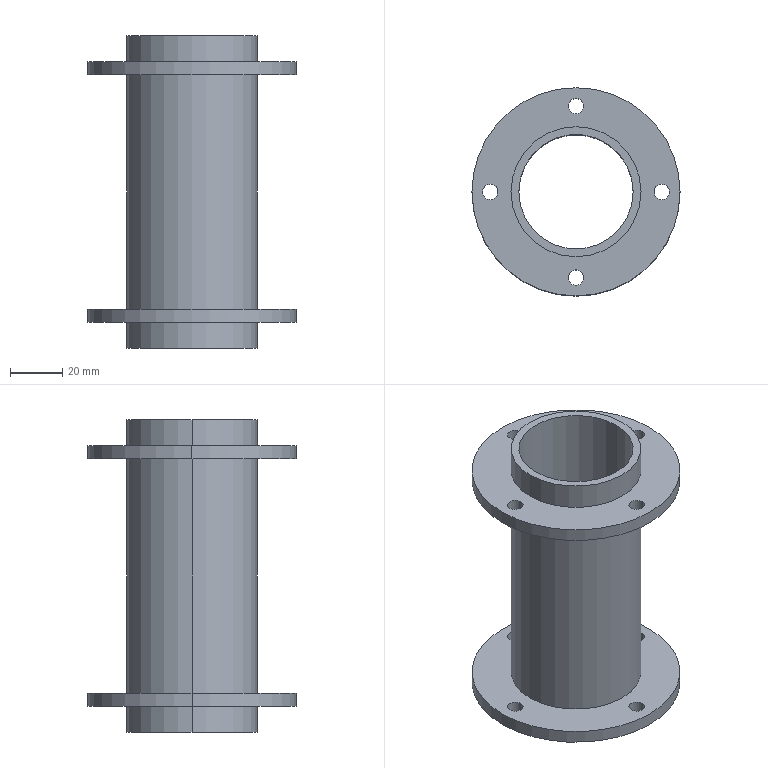Part | SolidWorks | features Extrusion 1, ICE 1, MirrorPattern 1 | 1 solid | 34 faces | box 80 x 80 x 120 mm | volume 82655 mm3 | cylinder 28 | plane 6 | commonest cylinder face diameters 6 x16 50 x6 80 x4 44 x2
STEP:
#1=CARTESIAN_POINT('',(36.,0.,45.));
#2=VERTEX_POINT('',#1);
#3=CARTESIAN_POINT('',(30.,0.,45.));
#4=VERTEX_POINT('',#3);
#5=CARTESIAN_POINT('',(33.,0.,45.));
#6=DIRECTION('',(0.,0.,-1.));
#7=DIRECTION('',(-1.,0.,0.));
#8=AXIS2_PLACEMENT_3D('',#5,#6,#7);
#9=CIRCLE('',#8,3.);
#10=EDGE_CURVE('',#2,#4,#9,.T.);
#11=ORIENTED_EDGE('',*,*,#10,.T.);
#12=CARTESIAN_POINT('',(30.,0.,50.));
#13=VERTEX_POINT('',#12);
#14=CARTESIAN_POINT('',(30.,0.,45.));
#15=DIRECTION('',(0.,0.,1.));
#16=VECTOR('',#15,1000.);
#17=LINE('',#14,#16);
#18=EDGE_CURVE('',#4,#13,#17,.T.);
#19=ORIENTED_EDGE('',*,*,#18,.T.);
#20=CARTESIAN_POINT('',(36.,0.,50.));
#21=VERTEX_POINT('',#20);
#22=CARTESIAN_POINT('',(33.,0.,50.));
#23=DIRECTION('',(0.,0.,-1.));
#24=DIRECTION('',(-1.,0.,0.));
#25=AXIS2_PLACEMENT_3D('',#22,#23,#24);
#26=CIRCLE('',#25,3.);
#27=EDGE_CURVE('',#21,#13,#26,.T.);
#28=ORIENTED_EDGE('',*,*,#27,.F.);
#29=CARTESIAN_POINT('',(36.,0.,45.));
#30=DIRECTION('',(0.,0.,1.));
#31=VECTOR('',#30,1000.);
#32=LINE('',#29,#31);
#33=EDGE_CURVE('',#2,#21,#32,.T.);
#34=ORIENTED_EDGE('',*,*,#33,.F.);
#35=EDGE_LOOP('',(#11,#19,#28,#34));
#36=FACE_OUTER_BOUND('',#35,.T.);
#37=CARTESIAN_POINT('',(33.,0.,45.));
#38=DIRECTION('',(0.,0.,1.));
#39=DIRECTION('',(1.,0.,0.));
#40=AXIS2_PLACEMENT_3D('',#37,#38,#39);
#41=CYLINDRICAL_SURFACE('',#40,3.);
#42=ADVANCED_FACE('',(#36),#41,.F.);
#43=CARTESIAN_POINT('',(3.,-33.,45.));
#44=VERTEX_POINT('',#43);
#45=CARTESIAN_POINT('',(-3.,-33.,45.));
#46=VERTEX_POINT('',#45);
#47=CARTESIAN_POINT('',(0.,-33.,45.));
#48=DIRECTION('',(0.,0.,-1.));
#49=DIRECTION('',(-1.,0.,0.));
#50=AXIS2_PLACEMENT_3D('',#47,#48,#49);
#51=CIRCLE('',#50,3.);
#52=EDGE_CURVE('',#44,#46,#51,.T.);
#53=ORIENTED_EDGE('',*,*,#52,.T.);
#54=CARTESIAN_POINT('',(-3.,-33.,50.));
#55=VERTEX_POINT('',#54);
#56=CARTESIAN_POINT('',(-3.,-33.,45.));
#57=DIRECTION('',(0.,0.,1.));
#58=VECTOR('',#57,1000.);
#59=LINE('',#56,#58);
#60=EDGE_CURVE('',#46,#55,#59,.T.);
#61=ORIENTED_EDGE('',*,*,#60,.T.);
#62=CARTESIAN_POINT('',(3.,-33.,50.));
#63=VERTEX_POINT('',#62);
#64=CARTESIAN_POINT('',(0.,-33.,50.));
#65=DIRECTION('',(0.,0.,-1.));
#66=DIRECTION('',(-1.,0.,0.));
#67=AXIS2_PLACEMENT_3D('',#64,#65,#66);
#68=CIRCLE('',#67,3.);
#69=EDGE_CURVE('',#63,#55,#68,.T.);
#70=ORIENTED_EDGE('',*,*,#69,.F.);
#71=CARTESIAN_POINT('',(3.,-33.,45.));
#72=DIRECTION('',(0.,0.,1.));
#73=VECTOR('',#72,1000.);
#74=LINE('',#71,#73);
#75=EDGE_CURVE('',#44,#63,#74,.T.);
#76=ORIENTED_EDGE('',*,*,#75,.F.);
#77=EDGE_LOOP('',(#53,#61,#70,#76));
#78=FACE_OUTER_BOUND('',#77,.T.);
#79=CARTESIAN_POINT('',(0.,-33.,45.));
#80=DIRECTION('',(0.,0.,1.));
#81=DIRECTION('',(1.,0.,0.));
#82=AXIS2_PLACEMENT_3D('',#79,#80,#81);
#83=CYLINDRICAL_SURFACE('',#82,3.);
#84=ADVANCED_FACE('',(#78),#83,.F.);
#85=CARTESIAN_POINT('',(-30.,0.,45.));
#86=VERTEX_POINT('',#85);
#87=CARTESIAN_POINT('',(-36.,0.,45.));
#88=VERTEX_POINT('',#87);
#89=CARTESIAN_POINT('',(-33.,0.,45.));
#90=DIRECTION('',(0.,0.,-1.));
#91=DIRECTION('',(-1.,0.,0.));
#92=AXIS2_PLACEMENT_3D('',#89,#90,#91);
#93=CIRCLE('',#92,3.);
#94=EDGE_CURVE('',#86,#88,#93,.T.);
#95=ORIENTED_EDGE('',*,*,#94,.T.);
#96=CARTESIAN_POINT('',(-36.,0.,50.));
#97=VERTEX_POINT('',#96);
#98=CARTESIAN_POINT('',(-36.,0.,45.));
#99=DIRECTION('',(0.,0.,1.));
#100=VECTOR('',#99,1000.);
#101=LINE('',#98,#100);
#102=EDGE_CURVE('',#88,#97,#101,.T.);
#103=ORIENTED_EDGE('',*,*,#102,.T.);
#104=CARTESIAN_POINT('',(-30.,0.,50.));
#105=VERTEX_POINT('',#104);
#106=CARTESIAN_POINT('',(-33.,0.,50.));
#107=DIRECTION('',(0.,0.,-1.));
#108=DIRECTION('',(-1.,0.,0.));
#109=AXIS2_PLACEMENT_3D('',#106,#107,#108);
#110=CIRCLE('',#109,3.);
#111=EDGE_CURVE('',#105,#97,#110,.T.);
#112=ORIENTED_EDGE('',*,*,#111,.F.);
#113=CARTESIAN_POINT('',(-30.,0.,45.));
#114=DIRECTION('',(0.,0.,1.));
#115=VECTOR('',#114,1000.);
#116=LINE('',#113,#115);
#117=EDGE_CURVE('',#86,#105,#116,.T.);
#118=ORIENTED_EDGE('',*,*,#117,.F.);
#119=EDGE_LOOP('',(#95,#103,#112,#118));
#120=FACE_OUTER_BOUND('',#119,.T.);
#121=CARTESIAN_POINT('',(-33.,0.,45.));
#122=DIRECTION('',(0.,0.,1.));
#123=DIRECTION('',(1.,0.,0.));
#124=AXIS2_PLACEMENT_3D('',#121,#122,#123);
#125=CYLINDRICAL_SURFACE('',#124,3.);
#126=ADVANCED_FACE('',(#120),#125,.F.);
#127=CARTESIAN_POINT('',(3.,33.,45.));
#128=VERTEX_POINT('',#127);
#129=CARTESIAN_POINT('',(-3.,33.,45.));
#130=VERTEX_POINT('',#129);
#131=CARTESIAN_POINT('',(0.,33.,45.));
#132=DIRECTION('',(0.,0.,-1.));
#133=DIRECTION('',(-1.,0.,0.));
#134=AXIS2_PLACEMENT_3D('',#131,#132,#133);
#135=CIRCLE('',#134,3.);
#136=EDGE_CURVE('',#128,#130,#135,.T.);
#137=ORIENTED_EDGE('',*,*,#136,.T.);
#138=CARTESIAN_POINT('',(-3.,33.,50.));
#139=VERTEX_POINT('',#138);
#140=CARTESIAN_POINT('',(-3.,33.,45.));
#141=DIRECTION('',(0.,0.,1.));
#142=VECTOR('',#141,1000.);
#143=LINE('',#140,#142);
#144=EDGE_CURVE('',#130,#139,#143,.T.);
#145=ORIENTED_EDGE('',*,*,#144,.T.);
#146=CARTESIAN_POINT('',(3.,33.,50.));
#147=VERTEX_POINT('',#146);
#148=CARTESIAN_POINT('',(0.,33.,50.));
#149=DIRECTION('',(0.,0.,-1.));
#150=DIRECTION('',(-1.,0.,0.));
#151=AXIS2_PLACEMENT_3D('',#148,#149,#150);
#152=CIRCLE('',#151,3.);
#153=EDGE_CURVE('',#147,#139,#152,.T.);
#154=ORIENTED_EDGE('',*,*,#153,.F.);
#155=CARTESIAN_POINT('',(3.,33.,45.));
#156=DIRECTION('',(0.,0.,1.));
#157=VECTOR('',#156,1000.);
#158=LINE('',#155,#157);
#159=EDGE_CURVE('',#128,#147,#158,.T.);
#160=ORIENTED_EDGE('',*,*,#159,.F.);
#161=EDGE_LOOP('',(#137,#145,#154,#160));
#162=FACE_OUTER_BOUND('',#161,.T.);
#163=CARTESIAN_POINT('',(0.,33.,45.));
#164=DIRECTION('',(0.,0.,1.));
#165=DIRECTION('',(1.,0.,0.));
#166=AXIS2_PLACEMENT_3D('',#163,#164,#165);
#167=CYLINDRICAL_SURFACE('',#166,3.);
#168=ADVANCED_FACE('',(#162),#167,.F.);
#169=CARTESIAN_POINT('',(-40.,0.,45.));
#170=VERTEX_POINT('',#169);
#171=CARTESIAN_POINT('',(40.,0.,45.));
#172=VERTEX_POINT('',#171);
#173=CARTESIAN_POINT('',(0.,0.,45.));
#174=DIRECTION('',(0.,0.,-1.));
#175=DIRECTION('',(-1.,0.,0.));
#176=AXIS2_PLACEMENT_3D('',#173,#174,#175);
#177=CIRCLE('',#176,40.);
#178=EDGE_CURVE('',#170,#172,#177,.T.);
#179=ORIENTED_EDGE('',*,*,#178,.F.);
#180=CARTESIAN_POINT('',(-40.,0.,50.));
#181=VERTEX_POINT('',#180);
#182=CARTESIAN_POINT('',(-40.,0.,45.));
#183=DIRECTION('',(0.,0.,1.));
#184=VECTOR('',#183,1000.);
#185=LINE('',#182,#184);
#186=EDGE_CURVE('',#170,#181,#185,.T.);
#187=ORIENTED_EDGE('',*,*,#186,.T.);
#188=CARTESIAN_POINT('',(40.,0.,50.));
#189=VERTEX_POINT('',#188);
#190=CARTESIAN_POINT('',(0.,0.,50.));
#191=DIRECTION('',(0.,0.,-1.));
#192=DIRECTION('',(-1.,0.,0.));
#193=AXIS2_PLACEMENT_3D('',#190,#191,#192);
#194=CIRCLE('',#193,40.);
#195=EDGE_CURVE('',#181,#189,#194,.T.);
#196=ORIENTED_EDGE('',*,*,#195,.T.);
#197=CARTESIAN_POINT('',(40.,0.,45.));
#198=DIRECTION('',(0.,0.,1.));
#199=VECTOR('',#198,1000.);
#200=LINE('',#197,#199);
#201=EDGE_CURVE('',#172,#189,#200,.T.);
#202=ORIENTED_EDGE('',*,*,#201,.F.);
#203=EDGE_LOOP('',(#179,#187,#196,#202));
#204=FACE_OUTER_BOUND('',#203,.T.);
#205=CARTESIAN_POINT('',(0.,0.,45.));
#206=DIRECTION('',(0.,0.,1.));
#207=DIRECTION('',(1.,0.,0.));
#208=AXIS2_PLACEMENT_3D('',#205,#206,#207);
#209=CYLINDRICAL_SURFACE('',#208,40.);
#210=ADVANCED_FACE('',(#204),#209,.T.);
#211=CARTESIAN_POINT('',(36.,0.,-45.));
#212=VERTEX_POINT('',#211);
#213=CARTESIAN_POINT('',(30.,0.,-45.));
#214=VERTEX_POINT('',#213);
#215=CARTESIAN_POINT('',(33.,0.,-45.));
#216=DIRECTION('',(0.,0.,-1.));
#217=DIRECTION('',(-1.,0.,0.));
#218=AXIS2_PLACEMENT_3D('',#215,#216,#217);
#219=CIRCLE('',#218,3.);
#220=EDGE_CURVE('',#212,#214,#219,.T.);
#221=ORIENTED_EDGE('',*,*,#220,.F.);
#222=CARTESIAN_POINT('',(36.,0.,-50.));
#223=VERTEX_POINT('',#222);
#224=CARTESIAN_POINT('',(36.,0.,-45.));
#225=DIRECTION('',(0.,0.,-1.));
#226=VECTOR('',#225,1000.);
#227=LINE('',#224,#226);
#228=EDGE_CURVE('',#212,#223,#227,.T.);
#229=ORIENTED_EDGE('',*,*,#228,.T.);
#230=CARTESIAN_POINT('',(30.,0.,-50.));
#231=VERTEX_POINT('',#230);
#232=CARTESIAN_POINT('',(33.,0.,-50.));
#233=DIRECTION('',(0.,0.,-1.));
#234=DIRECTION('',(-1.,0.,0.));
#235=AXIS2_PLACEMENT_3D('',#232,#233,#234);
#236=CIRCLE('',#235,3.);
#237=EDGE_CURVE('',#223,#231,#236,.T.);
#238=ORIENTED_EDGE('',*,*,#237,.T.);
#239=CARTESIAN_POINT('',(30.,0.,-45.));
#240=DIRECTION('',(0.,0.,-1.));
#241=VECTOR('',#240,1000.);
#242=LINE('',#239,#241);
#243=EDGE_CURVE('',#214,#231,#242,.T.);
#244=ORIENTED_EDGE('',*,*,#243,.F.);
#245=EDGE_LOOP('',(#221,#229,#238,#244));
#246=FACE_OUTER_BOUND('',#245,.T.);
#247=CARTESIAN_POINT('',(33.,0.,-45.));
#248=DIRECTION('',(0.,0.,-1.));
#249=DIRECTION('',(-1.,0.,0.));
#250=AXIS2_PLACEMENT_3D('',#247,#248,#249);
#251=CYLINDRICAL_SURFACE('',#250,3.);
#252=ADVANCED_FACE('',(#246),#251,.F.);
#253=CARTESIAN_POINT('',(3.,-33.,-45.));
#254=VERTEX_POINT('',#253);
#255=CARTESIAN_POINT('',(-3.,-33.,-45.));
#256=VERTEX_POINT('',#255);
#257=CARTESIAN_POINT('',(0.,-33.,-45.));
#258=DIRECTION('',(0.,0.,-1.));
#259=DIRECTION('',(-1.,0.,0.));
#260=AXIS2_PLACEMENT_3D('',#257,#258,#259);
#261=CIRCLE('',#260,3.);
#262=EDGE_CURVE('',#254,#256,#261,.T.);
#263=ORIENTED_EDGE('',*,*,#262,.F.);
#264=CARTESIAN_POINT('',(3.,-33.,-50.));
#265=VERTEX_POINT('',#264);
#266=CARTESIAN_POINT('',(3.,-33.,-45.));
#267=DIRECTION('',(0.,0.,-1.));
#268=VECTOR('',#267,1000.);
#269=LINE('',#266,#268);
#270=EDGE_CURVE('',#254,#265,#269,.T.);
#271=ORIENTED_EDGE('',*,*,#270,.T.);
#272=CARTESIAN_POINT('',(-3.,-33.,-50.));
#273=VERTEX_POINT('',#272);
#274=CARTESIAN_POINT('',(0.,-33.,-50.));
#275=DIRECTION('',(0.,0.,-1.));
#276=DIRECTION('',(-1.,0.,0.));
#277=AXIS2_PLACEMENT_3D('',#274,#275,#276);
#278=CIRCLE('',#277,3.);
#279=EDGE_CURVE('',#265,#273,#278,.T.);
#280=ORIENTED_EDGE('',*,*,#279,.T.);
#281=CARTESIAN_POINT('',(-3.,-33.,-45.));
#282=DIRECTION('',(0.,0.,-1.));
#283=VECTOR('',#282,1000.);
#284=LINE('',#281,#283);
#285=EDGE_CURVE('',#256,#273,#284,.T.);
#286=ORIENTED_EDGE('',*,*,#285,.F.);
#287=EDGE_LOOP('',(#263,#271,#280,#286));
#288=FACE_OUTER_BOUND('',#287,.T.);
#289=CARTESIAN_POINT('',(0.,-33.,-45.));
#290=DIRECTION('',(0.,0.,-1.));
#291=DIRECTION('',(-1.,0.,0.));
#292=AXIS2_PLACEMENT_3D('',#289,#290,#291);
#293=CYLINDRICAL_SURFACE('',#292,3.);
#294=ADVANCED_FACE('',(#288),#293,.F.);
#295=CARTESIAN_POINT('',(-30.,0.,-45.));
#296=VERTEX_POINT('',#295);
#297=CARTESIAN_POINT('',(-36.,0.,-45.));
#298=VERTEX_POINT('',#297);
#299=CARTESIAN_POINT('',(-33.,0.,-45.));
#300=DIRECTION('',(0.,0.,-1.));
#301=DIRECTION('',(-1.,0.,0.));
#302=AXIS2_PLACEMENT_3D('',#299,#300,#301);
#303=CIRCLE('',#302,3.);
#304=EDGE_CURVE('',#296,#298,#303,.T.);
#305=ORIENTED_EDGE('',*,*,#304,.F.);
#306=CARTESIAN_POINT('',(-30.,0.,-50.));
#307=VERTEX_POINT('',#306);
#308=CARTESIAN_POINT('',(-30.,0.,-45.));
#309=DIRECTION('',(0.,0.,-1.));
#310=VECTOR('',#309,1000.);
#311=LINE('',#308,#310);
#312=EDGE_CURVE('',#296,#307,#311,.T.);
#313=ORIENTED_EDGE('',*,*,#312,.T.);
#314=CARTESIAN_POINT('',(-36.,0.,-50.));
#315=VERTEX_POINT('',#314);
#316=CARTESIAN_POINT('',(-33.,0.,-50.));
#317=DIRECTION('',(0.,0.,-1.));
#318=DIRECTION('',(-1.,0.,0.));
#319=AXIS2_PLACEMENT_3D('',#316,#317,#318);
#320=CIRCLE('',#319,3.);
#321=EDGE_CURVE('',#307,#315,#320,.T.);
#322=ORIENTED_EDGE('',*,*,#321,.T.);
#323=CARTESIAN_POINT('',(-36.,0.,-45.));
#324=DIRECTION('',(0.,0.,-1.));
#325=VECTOR('',#324,1000.);
#326=LINE('',#323,#325);
#327=EDGE_CURVE('',#298,#315,#326,.T.);
#328=ORIENTED_EDGE('',*,*,#327,.F.);
#329=EDGE_LOOP('',(#305,#313,#322,#328));
#330=FACE_OUTER_BOUND('',#329,.T.);
#331=CARTESIAN_POINT('',(-33.,0.,-45.));
#332=DIRECTION('',(0.,0.,-1.));
#333=DIRECTION('',(-1.,0.,0.));
#334=AXIS2_PLACEMENT_3D('',#331,#332,#333);
#335=CYLINDRICAL_SURFACE('',#334,3.);
#336=ADVANCED_FACE('',(#330),#335,.F.);
#337=CARTESIAN_POINT('',(3.,33.,-45.));
#338=VERTEX_POINT('',#337);
#339=CARTESIAN_POINT('',(-3.,33.,-45.));
#340=VERTEX_POINT('',#339);
#341=CARTESIAN_POINT('',(0.,33.,-45.));
#342=DIRECTION('',(0.,0.,-1.));
#343=DIRECTION('',(-1.,0.,0.));
#344=AXIS2_PLACEMENT_3D('',#341,#342,#343);
#345=CIRCLE('',#344,3.);
#346=EDGE_CURVE('',#338,#340,#345,.T.);
#347=ORIENTED_EDGE('',*,*,#346,.F.);
#348=CARTESIAN_POINT('',(3.,33.,-50.));
#349=VERTEX_POINT('',#348);
#350=CARTESIAN_POINT('',(3.,33.,-45.));
#351=DIRECTION('',(0.,0.,-1.));
#352=VECTOR('',#351,1000.);
#353=LINE('',#350,#352);
#354=EDGE_CURVE('',#338,#349,#353,.T.);
#355=ORIENTED_EDGE('',*,*,#354,.T.);
#356=CARTESIAN_POINT('',(-3.,33.,-50.));
#357=VERTEX_POINT('',#356);
#358=CARTESIAN_POINT('',(0.,33.,-50.));
#359=DIRECTION('',(0.,0.,-1.));
#360=DIRECTION('',(-1.,0.,0.));
#361=AXIS2_PLACEMENT_3D('',#358,#359,#360);
#362=CIRCLE('',#361,3.);
#363=EDGE_CURVE('',#349,#357,#362,.T.);
#364=ORIENTED_EDGE('',*,*,#363,.T.);
#365=CARTESIAN_POINT('',(-3.,33.,-45.));
#366=DIRECTION('',(0.,0.,-1.));
#367=VECTOR('',#366,1000.);
#368=LINE('',#365,#367);
#369=EDGE_CURVE('',#340,#357,#368,.T.);
#370=ORIENTED_EDGE('',*,*,#369,.F.);
#371=EDGE_LOOP('',(#347,#355,#364,#370));
#372=FACE_OUTER_BOUND('',#371,.T.);
#373=CARTESIAN_POINT('',(0.,33.,-45.));
#374=DIRECTION('',(0.,0.,-1.));
#375=DIRECTION('',(-1.,0.,0.));
#376=AXIS2_PLACEMENT_3D('',#373,#374,#375);
#377=CYLINDRICAL_SURFACE('',#376,3.);
#378=ADVANCED_FACE('',(#372),#377,.F.);
#379=CARTESIAN_POINT('',(-40.,0.,-45.));
#380=VERTEX_POINT('',#379);
#381=CARTESIAN_POINT('',(40.,0.,-45.));
#382=VERTEX_POINT('',#381);
#383=CARTESIAN_POINT('',(0.,0.,-45.));
#384=DIRECTION('',(0.,0.,-1.));
#385=DIRECTION('',(-1.,0.,0.));
#386=AXIS2_PLACEMENT_3D('',#383,#384,#385);
#387=CIRCLE('',#386,40.);
#388=EDGE_CURVE('',#380,#382,#387,.T.);
#389=ORIENTED_EDGE('',*,*,#388,.T.);
#390=CARTESIAN_POINT('',(40.,0.,-50.));
#391=VERTEX_POINT('',#390);
#392=CARTESIAN_POINT('',(40.,0.,-45.));
#393=DIRECTION('',(0.,0.,-1.));
#394=VECTOR('',#393,1000.);
#395=LINE('',#392,#394);
#396=EDGE_CURVE('',#382,#391,#395,.T.);
#397=ORIENTED_EDGE('',*,*,#396,.T.);
#398=CARTESIAN_POINT('',(-40.,0.,-50.));
#399=VERTEX_POINT('',#398);
#400=CARTESIAN_POINT('',(0.,0.,-50.));
#401=DIRECTION('',(0.,0.,-1.));
#402=DIRECTION('',(-1.,0.,0.));
#403=AXIS2_PLACEMENT_3D('',#400,#401,#402);
#404=CIRCLE('',#403,40.);
#405=EDGE_CURVE('',#399,#391,#404,.T.);
#406=ORIENTED_EDGE('',*,*,#405,.F.);
#407=CARTESIAN_POINT('',(-40.,0.,-45.));
#408=DIRECTION('',(0.,0.,-1.));
#409=VECTOR('',#408,1000.);
#410=LINE('',#407,#409);
#411=EDGE_CURVE('',#380,#399,#410,.T.);
#412=ORIENTED_EDGE('',*,*,#411,.F.);
#413=EDGE_LOOP('',(#389,#397,#406,#412));
#414=FACE_OUTER_BOUND('',#413,.T.);
#415=CARTESIAN_POINT('',(0.,0.,-45.));
#416=DIRECTION('',(0.,0.,-1.));
#417=DIRECTION('',(-1.,0.,0.));
#418=AXIS2_PLACEMENT_3D('',#415,#416,#417);
#419=CYLINDRICAL_SURFACE('',#418,40.);
#420=ADVANCED_FACE('',(#414),#419,.T.);
#421=CARTESIAN_POINT('',(-22.,0.,60.));
#422=VERTEX_POINT('',#421);
#423=CARTESIAN_POINT('',(22.,0.,60.));
#424=VERTEX_POINT('',#423);
#425=CARTESIAN_POINT('',(0.,0.,60.));
#426=DIRECTION('',(0.,0.,1.));
#427=DIRECTION('',(1.,0.,0.));
#428=AXIS2_PLACEMENT_3D('',#425,#426,#427);
#429=CIRCLE('',#428,22.);
#430=EDGE_CURVE('',#422,#424,#429,.T.);
#431=ORIENTED_EDGE('',*,*,#430,.T.);
#432=CARTESIAN_POINT('',(22.,0.,-60.));
#433=VERTEX_POINT('',#432);
#434=CARTESIAN_POINT('',(22.,0.,60.));
#435=DIRECTION('',(0.,0.,-1.));
#436=VECTOR('',#435,1000.);
#437=LINE('',#434,#436);
#438=EDGE_CURVE('',#424,#433,#437,.T.);
#439=ORIENTED_EDGE('',*,*,#438,.T.);
#440=CARTESIAN_POINT('',(-22.,0.,-60.));
#441=VERTEX_POINT('',#440);
#442=CARTESIAN_POINT('',(0.,0.,-60.));
#443=DIRECTION('',(0.,0.,1.));
#444=DIRECTION('',(1.,0.,0.));
#445=AXIS2_PLACEMENT_3D('',#442,#443,#444);
#446=CIRCLE('',#445,22.);
#447=EDGE_CURVE('',#441,#433,#446,.T.);
#448=ORIENTED_EDGE('',*,*,#447,.F.);
#449=CARTESIAN_POINT('',(-22.,0.,60.));
#450=DIRECTION('',(0.,0.,-1.));
#451=VECTOR('',#450,1000.);
#452=LINE('',#449,#451);
#453=EDGE_CURVE('',#422,#441,#452,.T.);
#454=ORIENTED_EDGE('',*,*,#453,.F.);
#455=EDGE_LOOP('',(#431,#439,#448,#454));
#456=FACE_OUTER_BOUND('',#455,.T.);
#457=CARTESIAN_POINT('',(0.,0.,60.));
#458=DIRECTION('',(0.,0.,-1.));
#459=DIRECTION('',(-1.,0.,0.));
#460=AXIS2_PLACEMENT_3D('',#457,#458,#459);
#461=CYLINDRICAL_SURFACE('',#460,22.);
#462=ADVANCED_FACE('',(#456),#461,.F.);
#463=CARTESIAN_POINT('',(-25.,0.,-50.));
#464=VERTEX_POINT('',#463);
#465=CARTESIAN_POINT('',(25.,0.,-50.));
#466=VERTEX_POINT('',#465);
#467=CARTESIAN_POINT('',(0.,0.,-50.));
#468=DIRECTION('',(0.,0.,-1.));
#469=DIRECTION('',(-1.,0.,0.));
#470=AXIS2_PLACEMENT_3D('',#467,#468,#469);
#471=CIRCLE('',#470,25.);
#472=EDGE_CURVE('',#464,#466,#471,.T.);
#473=ORIENTED_EDGE('',*,*,#472,.T.);
#474=CARTESIAN_POINT('',(25.,0.,-60.));
#475=VERTEX_POINT('',#474);
#476=CARTESIAN_POINT('',(25.,0.,60.));
#477=DIRECTION('',(0.,0.,-1.));
#478=VECTOR('',#477,1000.);
#479=LINE('',#476,#478);
#480=EDGE_CURVE('',#466,#475,#479,.T.);
#481=ORIENTED_EDGE('',*,*,#480,.T.);
#482=CARTESIAN_POINT('',(-25.,0.,-60.));
#483=VERTEX_POINT('',#482);
#484=CARTESIAN_POINT('',(0.,0.,-60.));
#485=DIRECTION('',(0.,0.,1.));
#486=DIRECTION('',(1.,0.,0.));
#487=AXIS2_PLACEMENT_3D('',#484,#485,#486);
#488=CIRCLE('',#487,25.);
#489=EDGE_CURVE('',#475,#483,#488,.T.);
#490=ORIENTED_EDGE('',*,*,#489,.T.);
#491=CARTESIAN_POINT('',(-25.,0.,60.));
#492=DIRECTION('',(0.,0.,-1.));
#493=VECTOR('',#492,1000.);
#494=LINE('',#491,#493);
#495=EDGE_CURVE('',#464,#483,#494,.T.);
#496=ORIENTED_EDGE('',*,*,#495,.F.);
#497=EDGE_LOOP('',(#473,#481,#490,#496));
#498=FACE_OUTER_BOUND('',#497,.T.);
#499=CARTESIAN_POINT('',(0.,0.,60.));
#500=DIRECTION('',(0.,0.,-1.));
#501=DIRECTION('',(-1.,0.,0.));
#502=AXIS2_PLACEMENT_3D('',#499,#500,#501);
#503=CYLINDRICAL_SURFACE('',#502,25.);
#504=ADVANCED_FACE('',(#498),#503,.T.);
#505=CARTESIAN_POINT('',(25.,0.,60.));
#506=VERTEX_POINT('',#505);
#507=CARTESIAN_POINT('',(-25.,0.,60.));
#508=VERTEX_POINT('',#507);
#509=CARTESIAN_POINT('',(0.,0.,60.));
#510=DIRECTION('',(0.,0.,1.));
#511=DIRECTION('',(1.,0.,0.));
#512=AXIS2_PLACEMENT_3D('',#509,#510,#511);
#513=CIRCLE('',#512,25.);
#514=EDGE_CURVE('',#506,#508,#513,.T.);
#515=ORIENTED_EDGE('',*,*,#514,.F.);
#516=CARTESIAN_POINT('',(25.,0.,50.));
#517=VERTEX_POINT('',#516);
#518=CARTESIAN_POINT('',(25.,0.,60.));
#519=DIRECTION('',(0.,0.,-1.));
#520=VECTOR('',#519,1000.);
#521=LINE('',#518,#520);
#522=EDGE_CURVE('',#506,#517,#521,.T.);
#523=ORIENTED_EDGE('',*,*,#522,.T.);
#524=CARTESIAN_POINT('',(-25.,0.,50.));
#525=VERTEX_POINT('',#524);
#526=CARTESIAN_POINT('',(0.,0.,50.));
#527=DIRECTION('',(0.,0.,-1.));
#528=DIRECTION('',(-1.,0.,0.));
#529=AXIS2_PLACEMENT_3D('',#526,#527,#528);
#530=CIRCLE('',#529,25.);
#531=EDGE_CURVE('',#525,#517,#530,.T.);
#532=ORIENTED_EDGE('',*,*,#531,.F.);
#533=CARTESIAN_POINT('',(-25.,0.,60.));
#534=DIRECTION('',(0.,0.,-1.));
#535=VECTOR('',#534,1000.);
#536=LINE('',#533,#535);
#537=EDGE_CURVE('',#508,#525,#536,.T.);
#538=ORIENTED_EDGE('',*,*,#537,.F.);
#539=EDGE_LOOP('',(#515,#523,#532,#538));
#540=FACE_OUTER_BOUND('',#539,.T.);
#541=CARTESIAN_POINT('',(0.,0.,60.));
#542=DIRECTION('',(0.,0.,-1.));
#543=DIRECTION('',(-1.,0.,0.));
#544=AXIS2_PLACEMENT_3D('',#541,#542,#543);
#545=CYLINDRICAL_SURFACE('',#544,25.);
#546=ADVANCED_FACE('',(#540),#545,.T.);
#547=CARTESIAN_POINT('',(25.,0.,45.));
#548=VERTEX_POINT('',#547);
#549=CARTESIAN_POINT('',(-25.,0.,45.));
#550=VERTEX_POINT('',#549);
#551=CARTESIAN_POINT('',(0.,0.,45.));
#552=DIRECTION('',(0.,0.,1.));
#553=DIRECTION('',(1.,0.,0.));
#554=AXIS2_PLACEMENT_3D('',#551,#552,#553);
#555=CIRCLE('',#554,25.);
#556=EDGE_CURVE('',#548,#550,#555,.T.);
#557=ORIENTED_EDGE('',*,*,#556,.F.);
#558=CARTESIAN_POINT('',(25.,0.,-45.));
#559=VERTEX_POINT('',#558);
#560=CARTESIAN_POINT('',(25.,0.,60.));
#561=DIRECTION('',(0.,0.,-1.));
#562=VECTOR('',#561,1000.);
#563=LINE('',#560,#562);
#564=EDGE_CURVE('',#548,#559,#563,.T.);
#565=ORIENTED_EDGE('',*,*,#564,.T.);
#566=CARTESIAN_POINT('',(-25.,0.,-45.));
#567=VERTEX_POINT('',#566);
#568=CARTESIAN_POINT('',(0.,0.,-45.));
#569=DIRECTION('',(0.,0.,-1.));
#570=DIRECTION('',(-1.,0.,0.));
#571=AXIS2_PLACEMENT_3D('',#568,#569,#570);
#572=CIRCLE('',#571,25.);
#573=EDGE_CURVE('',#567,#559,#572,.T.);
#574=ORIENTED_EDGE('',*,*,#573,.F.);
#575=CARTESIAN_POINT('',(-25.,0.,60.));
#576=DIRECTION('',(0.,0.,-1.));
#577=VECTOR('',#576,1000.);
#578=LINE('',#575,#577);
#579=EDGE_CURVE('',#550,#567,#578,.T.);
#580=ORIENTED_EDGE('',*,*,#579,.F.);
#581=EDGE_LOOP('',(#557,#565,#574,#580));
#582=FACE_OUTER_BOUND('',#581,.T.);
#583=CARTESIAN_POINT('',(0.,0.,60.));
#584=DIRECTION('',(0.,0.,-1.));
#585=DIRECTION('',(-1.,0.,0.));
#586=AXIS2_PLACEMENT_3D('',#583,#584,#585);
#587=CYLINDRICAL_SURFACE('',#586,25.);
#588=ADVANCED_FACE('',(#582),#587,.T.);
#589=ORIENTED_EDGE('',*,*,#564,.F.);
#590=CARTESIAN_POINT('',(0.,0.,45.));
#591=DIRECTION('',(0.,0.,1.));
#592=DIRECTION('',(1.,0.,0.));
#593=AXIS2_PLACEMENT_3D('',#590,#591,#592);
#594=CIRCLE('',#593,25.);
#595=EDGE_CURVE('',#550,#548,#594,.T.);
#596=ORIENTED_EDGE('',*,*,#595,.F.);
#597=ORIENTED_EDGE('',*,*,#579,.T.);
#598=CARTESIAN_POINT('',(0.,0.,-45.));
#599=DIRECTION('',(0.,0.,-1.));
#600=DIRECTION('',(-1.,0.,0.));
#601=AXIS2_PLACEMENT_3D('',#598,#599,#600);
#602=CIRCLE('',#601,25.);
#603=EDGE_CURVE('',#559,#567,#602,.T.);
#604=ORIENTED_EDGE('',*,*,#603,.F.);
#605=EDGE_LOOP('',(#589,#596,#597,#604));
#606=FACE_OUTER_BOUND('',#605,.T.);
#607=CARTESIAN_POINT('',(0.,0.,60.));
#608=DIRECTION('',(0.,0.,-1.));
#609=DIRECTION('',(-1.,0.,0.));
#610=AXIS2_PLACEMENT_3D('',#607,#608,#609);
#611=CYLINDRICAL_SURFACE('',#610,25.);
#612=ADVANCED_FACE('',(#606),#611,.T.);
#613=ORIENTED_EDGE('',*,*,#522,.F.);
#614=CARTESIAN_POINT('',(0.,0.,60.));
#615=DIRECTION('',(0.,0.,1.));
#616=DIRECTION('',(1.,0.,0.));
#617=AXIS2_PLACEMENT_3D('',#614,#615,#616);
#618=CIRCLE('',#617,25.);
#619=EDGE_CURVE('',#508,#506,#618,.T.);
#620=ORIENTED_EDGE('',*,*,#619,.F.);
#621=ORIENTED_EDGE('',*,*,#537,.T.);
#622=CARTESIAN_POINT('',(0.,0.,50.));
#623=DIRECTION('',(0.,0.,-1.));
#624=DIRECTION('',(-1.,0.,0.));
#625=AXIS2_PLACEMENT_3D('',#622,#623,#624);
#626=CIRCLE('',#625,25.);
#627=EDGE_CURVE('',#517,#525,#626,.T.);
#628=ORIENTED_EDGE('',*,*,#627,.F.);
#629=EDGE_LOOP('',(#613,#620,#621,#628));
#630=FACE_OUTER_BOUND('',#629,.T.);
#631=CARTESIAN_POINT('',(0.,0.,60.));
#632=DIRECTION('',(0.,0.,-1.));
#633=DIRECTION('',(-1.,0.,0.));
#634=AXIS2_PLACEMENT_3D('',#631,#632,#633);
#635=CYLINDRICAL_SURFACE('',#634,25.);
#636=ADVANCED_FACE('',(#630),#635,.T.);
#637=ORIENTED_EDGE('',*,*,#619,.T.);
#638=ORIENTED_EDGE('',*,*,#514,.T.);
#639=EDGE_LOOP('',(#637,#638));
#640=FACE_OUTER_BOUND('',#639,.T.);
#641=ORIENTED_EDGE('',*,*,#430,.F.);
#642=CARTESIAN_POINT('',(0.,0.,60.));
#643=DIRECTION('',(0.,0.,1.));
#644=DIRECTION('',(1.,0.,0.));
#645=AXIS2_PLACEMENT_3D('',#642,#643,#644);
#646=CIRCLE('',#645,22.);
#647=EDGE_CURVE('',#424,#422,#646,.T.);
#648=ORIENTED_EDGE('',*,*,#647,.F.);
#649=EDGE_LOOP('',(#641,#648));
#650=FACE_BOUND('',#649,.T.);
#651=CARTESIAN_POINT('',(0.,0.,60.));
#652=DIRECTION('',(0.,0.,1.));
#653=DIRECTION('',(1.,0.,0.));
#654=AXIS2_PLACEMENT_3D('',#651,#652,#653);
#655=PLANE('',#654);
#656=ADVANCED_FACE('',(#640,#650),#655,.T.);
#657=CARTESIAN_POINT('',(0.,0.,-60.));
#658=DIRECTION('',(0.,0.,1.));
#659=DIRECTION('',(1.,0.,0.));
#660=AXIS2_PLACEMENT_3D('',#657,#658,#659);
#661=CIRCLE('',#660,25.);
#662=EDGE_CURVE('',#483,#475,#661,.T.);
#663=ORIENTED_EDGE('',*,*,#662,.F.);
#664=ORIENTED_EDGE('',*,*,#489,.F.);
#665=EDGE_LOOP('',(#663,#664));
#666=FACE_OUTER_BOUND('',#665,.T.);
#667=ORIENTED_EDGE('',*,*,#447,.T.);
#668=CARTESIAN_POINT('',(0.,0.,-60.));
#669=DIRECTION('',(0.,0.,1.));
#670=DIRECTION('',(1.,0.,0.));
#671=AXIS2_PLACEMENT_3D('',#668,#669,#670);
#672=CIRCLE('',#671,22.);
#673=EDGE_CURVE('',#433,#441,#672,.T.);
#674=ORIENTED_EDGE('',*,*,#673,.T.);
#675=EDGE_LOOP('',(#667,#674));
#676=FACE_BOUND('',#675,.T.);
#677=CARTESIAN_POINT('',(0.,0.,-60.));
#678=DIRECTION('',(0.,0.,1.));
#679=DIRECTION('',(1.,0.,0.));
#680=AXIS2_PLACEMENT_3D('',#677,#678,#679);
#681=PLANE('',#680);
#682=ADVANCED_FACE('',(#666,#676),#681,.F.);
#683=ORIENTED_EDGE('',*,*,#480,.F.);
#684=CARTESIAN_POINT('',(0.,0.,-50.));
#685=DIRECTION('',(0.,0.,-1.));
#686=DIRECTION('',(-1.,0.,0.));
#687=AXIS2_PLACEMENT_3D('',#684,#685,#686);
#688=CIRCLE('',#687,25.);
#689=EDGE_CURVE('',#466,#464,#688,.T.);
#690=ORIENTED_EDGE('',*,*,#689,.T.);
#691=ORIENTED_EDGE('',*,*,#495,.T.);
#692=ORIENTED_EDGE('',*,*,#662,.T.);
#693=EDGE_LOOP('',(#683,#690,#691,#692));
#694=FACE_OUTER_BOUND('',#693,.T.);
#695=CARTESIAN_POINT('',(0.,0.,60.));
#696=DIRECTION('',(0.,0.,-1.));
#697=DIRECTION('',(-1.,0.,0.));
#698=AXIS2_PLACEMENT_3D('',#695,#696,#697);
#699=CYLINDRICAL_SURFACE('',#698,25.);
#700=ADVANCED_FACE('',(#694),#699,.T.);
#701=ORIENTED_EDGE('',*,*,#438,.F.);
#702=ORIENTED_EDGE('',*,*,#647,.T.);
#703=ORIENTED_EDGE('',*,*,#453,.T.);
#704=ORIENTED_EDGE('',*,*,#673,.F.);
#705=EDGE_LOOP('',(#701,#702,#703,#704));
#706=FACE_OUTER_BOUND('',#705,.T.);
#707=CARTESIAN_POINT('',(0.,0.,60.));
#708=DIRECTION('',(0.,0.,-1.));
#709=DIRECTION('',(-1.,0.,0.));
#710=AXIS2_PLACEMENT_3D('',#707,#708,#709);
#711=CYLINDRICAL_SURFACE('',#710,22.);
#712=ADVANCED_FACE('',(#706),#711,.F.);
#713=ORIENTED_EDGE('',*,*,#396,.F.);
#714=CARTESIAN_POINT('',(0.,0.,-45.));
#715=DIRECTION('',(0.,0.,-1.));
#716=DIRECTION('',(-1.,0.,0.));
#717=AXIS2_PLACEMENT_3D('',#714,#715,#716);
#718=CIRCLE('',#717,40.);
#719=EDGE_CURVE('',#382,#380,#718,.T.);
#720=ORIENTED_EDGE('',*,*,#719,.T.);
#721=ORIENTED_EDGE('',*,*,#411,.T.);
#722=CARTESIAN_POINT('',(0.,0.,-50.));
#723=DIRECTION('',(0.,0.,-1.));
#724=DIRECTION('',(-1.,0.,0.));
#725=AXIS2_PLACEMENT_3D('',#722,#723,#724);
#726=CIRCLE('',#725,40.);
#727=EDGE_CURVE('',#391,#399,#726,.T.);
#728=ORIENTED_EDGE('',*,*,#727,.F.);
#729=EDGE_LOOP('',(#713,#720,#721,#728));
#730=FACE_OUTER_BOUND('',#729,.T.);
#731=CARTESIAN_POINT('',(0.,0.,-45.));
#732=DIRECTION('',(0.,0.,-1.));
#733=DIRECTION('',(-1.,0.,0.));
#734=AXIS2_PLACEMENT_3D('',#731,#732,#733);
#735=CYLINDRICAL_SURFACE('',#734,40.);
#736=ADVANCED_FACE('',(#730),#735,.T.);
#737=CARTESIAN_POINT('',(33.,0.,-45.));
#738=DIRECTION('',(0.,0.,-1.));
#739=DIRECTION('',(-1.,0.,0.));
#740=AXIS2_PLACEMENT_3D('',#737,#738,#739);
#741=CIRCLE('',#740,3.);
#742=EDGE_CURVE('',#214,#212,#741,.T.);
#743=ORIENTED_EDGE('',*,*,#742,.T.);
#744=ORIENTED_EDGE('',*,*,#220,.T.);
#745=EDGE_LOOP('',(#743,#744));
#746=FACE_BOUND('',#745,.T.);
#747=CARTESIAN_POINT('',(0.,-33.,-45.));
#748=DIRECTION('',(0.,0.,-1.));
#749=DIRECTION('',(-1.,0.,0.));
#750=AXIS2_PLACEMENT_3D('',#747,#748,#749);
#751=CIRCLE('',#750,3.);
#752=EDGE_CURVE('',#256,#254,#751,.T.);
#753=ORIENTED_EDGE('',*,*,#752,.T.);
#754=ORIENTED_EDGE('',*,*,#262,.T.);
#755=EDGE_LOOP('',(#753,#754));
#756=FACE_BOUND('',#755,.T.);
#757=CARTESIAN_POINT('',(-33.,0.,-45.));
#758=DIRECTION('',(0.,0.,-1.));
#759=DIRECTION('',(-1.,0.,0.));
#760=AXIS2_PLACEMENT_3D('',#757,#758,#759);
#761=CIRCLE('',#760,3.);
#762=EDGE_CURVE('',#298,#296,#761,.T.);
#763=ORIENTED_EDGE('',*,*,#762,.T.);
#764=ORIENTED_EDGE('',*,*,#304,.T.);
#765=EDGE_LOOP('',(#763,#764));
#766=FACE_BOUND('',#765,.T.);
#767=CARTESIAN_POINT('',(0.,33.,-45.));
#768=DIRECTION('',(0.,0.,-1.));
#769=DIRECTION('',(-1.,0.,0.));
#770=AXIS2_PLACEMENT_3D('',#767,#768,#769);
#771=CIRCLE('',#770,3.);
#772=EDGE_CURVE('',#340,#338,#771,.T.);
#773=ORIENTED_EDGE('',*,*,#772,.T.);
#774=ORIENTED_EDGE('',*,*,#346,.T.);
#775=EDGE_LOOP('',(#773,#774));
#776=FACE_BOUND('',#775,.T.);
#777=ORIENTED_EDGE('',*,*,#573,.T.);
#778=ORIENTED_EDGE('',*,*,#603,.T.);
#779=EDGE_LOOP('',(#777,#778));
#780=FACE_BOUND('',#779,.T.);
#781=ORIENTED_EDGE('',*,*,#388,.F.);
#782=ORIENTED_EDGE('',*,*,#719,.F.);
#783=EDGE_LOOP('',(#781,#782));
#784=FACE_OUTER_BOUND('',#783,.T.);
#785=CARTESIAN_POINT('',(0.,0.,-45.));
#786=DIRECTION('',(0.,0.,-1.));
#787=DIRECTION('',(-1.,0.,0.));
#788=AXIS2_PLACEMENT_3D('',#785,#786,#787);
#789=PLANE('',#788);
#790=ADVANCED_FACE('',(#746,#756,#766,#776,#780,#784),#789,.F.);
#791=CARTESIAN_POINT('',(33.,0.,-50.));
#792=DIRECTION('',(0.,0.,-1.));
#793=DIRECTION('',(-1.,0.,0.));
#794=AXIS2_PLACEMENT_3D('',#791,#792,#793);
#795=CIRCLE('',#794,3.);
#796=EDGE_CURVE('',#231,#223,#795,.T.);
#797=ORIENTED_EDGE('',*,*,#796,.F.);
#798=ORIENTED_EDGE('',*,*,#237,.F.);
#799=EDGE_LOOP('',(#797,#798));
#800=FACE_BOUND('',#799,.T.);
#801=CARTESIAN_POINT('',(0.,-33.,-50.));
#802=DIRECTION('',(0.,0.,-1.));
#803=DIRECTION('',(-1.,0.,0.));
#804=AXIS2_PLACEMENT_3D('',#801,#802,#803);
#805=CIRCLE('',#804,3.);
#806=EDGE_CURVE('',#273,#265,#805,.T.);
#807=ORIENTED_EDGE('',*,*,#806,.F.);
#808=ORIENTED_EDGE('',*,*,#279,.F.);
#809=EDGE_LOOP('',(#807,#808));
#810=FACE_BOUND('',#809,.T.);
#811=CARTESIAN_POINT('',(-33.,0.,-50.));
#812=DIRECTION('',(0.,0.,-1.));
#813=DIRECTION('',(-1.,0.,0.));
#814=AXIS2_PLACEMENT_3D('',#811,#812,#813);
#815=CIRCLE('',#814,3.);
#816=EDGE_CURVE('',#315,#307,#815,.T.);
#817=ORIENTED_EDGE('',*,*,#816,.F.);
#818=ORIENTED_EDGE('',*,*,#321,.F.);
#819=EDGE_LOOP('',(#817,#818));
#820=FACE_BOUND('',#819,.T.);
#821=CARTESIAN_POINT('',(0.,33.,-50.));
#822=DIRECTION('',(0.,0.,-1.));
#823=DIRECTION('',(-1.,0.,0.));
#824=AXIS2_PLACEMENT_3D('',#821,#822,#823);
#825=CIRCLE('',#824,3.);
#826=EDGE_CURVE('',#357,#349,#825,.T.);
#827=ORIENTED_EDGE('',*,*,#826,.F.);
#828=ORIENTED_EDGE('',*,*,#363,.F.);
#829=EDGE_LOOP('',(#827,#828));
#830=FACE_BOUND('',#829,.T.);
#831=ORIENTED_EDGE('',*,*,#472,.F.);
#832=ORIENTED_EDGE('',*,*,#689,.F.);
#833=EDGE_LOOP('',(#831,#832));
#834=FACE_BOUND('',#833,.T.);
#835=ORIENTED_EDGE('',*,*,#405,.T.);
#836=ORIENTED_EDGE('',*,*,#727,.T.);
#837=EDGE_LOOP('',(#835,#836));
#838=FACE_OUTER_BOUND('',#837,.T.);
#839=CARTESIAN_POINT('',(0.,0.,-50.));
#840=DIRECTION('',(0.,0.,-1.));
#841=DIRECTION('',(-1.,0.,0.));
#842=AXIS2_PLACEMENT_3D('',#839,#840,#841);
#843=PLANE('',#842);
#844=ADVANCED_FACE('',(#800,#810,#820,#830,#834,#838),#843,.T.);
#845=ORIENTED_EDGE('',*,*,#354,.F.);
#846=ORIENTED_EDGE('',*,*,#772,.F.);
#847=ORIENTED_EDGE('',*,*,#369,.T.);
#848=ORIENTED_EDGE('',*,*,#826,.T.);
#849=EDGE_LOOP('',(#845,#846,#847,#848));
#850=FACE_OUTER_BOUND('',#849,.T.);
#851=CARTESIAN_POINT('',(0.,33.,-45.));
#852=DIRECTION('',(0.,0.,-1.));
#853=DIRECTION('',(-1.,0.,0.));
#854=AXIS2_PLACEMENT_3D('',#851,#852,#853);
#855=CYLINDRICAL_SURFACE('',#854,3.);
#856=ADVANCED_FACE('',(#850),#855,.F.);
#857=ORIENTED_EDGE('',*,*,#312,.F.);
#858=ORIENTED_EDGE('',*,*,#762,.F.);
#859=ORIENTED_EDGE('',*,*,#327,.T.);
#860=ORIENTED_EDGE('',*,*,#816,.T.);
#861=EDGE_LOOP('',(#857,#858,#859,#860));
#862=FACE_OUTER_BOUND('',#861,.T.);
#863=CARTESIAN_POINT('',(-33.,0.,-45.));
#864=DIRECTION('',(0.,0.,-1.));
#865=DIRECTION('',(-1.,0.,0.));
#866=AXIS2_PLACEMENT_3D('',#863,#864,#865);
#867=CYLINDRICAL_SURFACE('',#866,3.);
#868=ADVANCED_FACE('',(#862),#867,.F.);
#869=ORIENTED_EDGE('',*,*,#270,.F.);
#870=ORIENTED_EDGE('',*,*,#752,.F.);
#871=ORIENTED_EDGE('',*,*,#285,.T.);
#872=ORIENTED_EDGE('',*,*,#806,.T.);
#873=EDGE_LOOP('',(#869,#870,#871,#872));
#874=FACE_OUTER_BOUND('',#873,.T.);
#875=CARTESIAN_POINT('',(0.,-33.,-45.));
#876=DIRECTION('',(0.,0.,-1.));
#877=DIRECTION('',(-1.,0.,0.));
#878=AXIS2_PLACEMENT_3D('',#875,#876,#877);
#879=CYLINDRICAL_SURFACE('',#878,3.);
#880=ADVANCED_FACE('',(#874),#879,.F.);
#881=ORIENTED_EDGE('',*,*,#228,.F.);
#882=ORIENTED_EDGE('',*,*,#742,.F.);
#883=ORIENTED_EDGE('',*,*,#243,.T.);
#884=ORIENTED_EDGE('',*,*,#796,.T.);
#885=EDGE_LOOP('',(#881,#882,#883,#884));
#886=FACE_OUTER_BOUND('',#885,.T.);
#887=CARTESIAN_POINT('',(33.,0.,-45.));
#888=DIRECTION('',(0.,0.,-1.));
#889=DIRECTION('',(-1.,0.,0.));
#890=AXIS2_PLACEMENT_3D('',#887,#888,#889);
#891=CYLINDRICAL_SURFACE('',#890,3.);
#892=ADVANCED_FACE('',(#886),#891,.F.);
#893=CARTESIAN_POINT('',(0.,0.,45.));
#894=DIRECTION('',(0.,0.,-1.));
#895=DIRECTION('',(-1.,0.,0.));
#896=AXIS2_PLACEMENT_3D('',#893,#894,#895);
#897=CIRCLE('',#896,40.);
#898=EDGE_CURVE('',#172,#170,#897,.T.);
#899=ORIENTED_EDGE('',*,*,#898,.T.);
#900=ORIENTED_EDGE('',*,*,#178,.T.);
#901=EDGE_LOOP('',(#899,#900));
#902=FACE_OUTER_BOUND('',#901,.T.);
#903=ORIENTED_EDGE('',*,*,#595,.T.);
#904=ORIENTED_EDGE('',*,*,#556,.T.);
#905=EDGE_LOOP('',(#903,#904));
#906=FACE_BOUND('',#905,.T.);
#907=ORIENTED_EDGE('',*,*,#136,.F.);
#908=CARTESIAN_POINT('',(0.,33.,45.));
#909=DIRECTION('',(0.,0.,-1.));
#910=DIRECTION('',(-1.,0.,0.));
#911=AXIS2_PLACEMENT_3D('',#908,#909,#910);
#912=CIRCLE('',#911,3.);
#913=EDGE_CURVE('',#130,#128,#912,.T.);
#914=ORIENTED_EDGE('',*,*,#913,.F.);
#915=EDGE_LOOP('',(#907,#914));
#916=FACE_BOUND('',#915,.T.);
#917=ORIENTED_EDGE('',*,*,#94,.F.);
#918=CARTESIAN_POINT('',(-33.,0.,45.));
#919=DIRECTION('',(0.,0.,-1.));
#920=DIRECTION('',(-1.,0.,0.));
#921=AXIS2_PLACEMENT_3D('',#918,#919,#920);
#922=CIRCLE('',#921,3.);
#923=EDGE_CURVE('',#88,#86,#922,.T.);
#924=ORIENTED_EDGE('',*,*,#923,.F.);
#925=EDGE_LOOP('',(#917,#924));
#926=FACE_BOUND('',#925,.T.);
#927=ORIENTED_EDGE('',*,*,#52,.F.);
#928=CARTESIAN_POINT('',(0.,-33.,45.));
#929=DIRECTION('',(0.,0.,-1.));
#930=DIRECTION('',(-1.,0.,0.));
#931=AXIS2_PLACEMENT_3D('',#928,#929,#930);
#932=CIRCLE('',#931,3.);
#933=EDGE_CURVE('',#46,#44,#932,.T.);
#934=ORIENTED_EDGE('',*,*,#933,.F.);
#935=EDGE_LOOP('',(#927,#934));
#936=FACE_BOUND('',#935,.T.);
#937=ORIENTED_EDGE('',*,*,#10,.F.);
#938=CARTESIAN_POINT('',(33.,0.,45.));
#939=DIRECTION('',(0.,0.,-1.));
#940=DIRECTION('',(-1.,0.,0.));
#941=AXIS2_PLACEMENT_3D('',#938,#939,#940);
#942=CIRCLE('',#941,3.);
#943=EDGE_CURVE('',#4,#2,#942,.T.);
#944=ORIENTED_EDGE('',*,*,#943,.F.);
#945=EDGE_LOOP('',(#937,#944));
#946=FACE_BOUND('',#945,.T.);
#947=CARTESIAN_POINT('',(0.,0.,45.));
#948=DIRECTION('',(0.,0.,1.));
#949=DIRECTION('',(-1.,0.,0.));
#950=AXIS2_PLACEMENT_3D('',#947,#948,#949);
#951=PLANE('',#950);
#952=ADVANCED_FACE('',(#902,#906,#916,#926,#936,#946),#951,.F.);
#953=ORIENTED_EDGE('',*,*,#69,.T.);
#954=CARTESIAN_POINT('',(0.,-33.,50.));
#955=DIRECTION('',(0.,0.,-1.));
#956=DIRECTION('',(-1.,0.,0.));
#957=AXIS2_PLACEMENT_3D('',#954,#955,#956);
#958=CIRCLE('',#957,3.);
#959=EDGE_CURVE('',#55,#63,#958,.T.);
#960=ORIENTED_EDGE('',*,*,#959,.T.);
#961=EDGE_LOOP('',(#953,#960));
#962=FACE_BOUND('',#961,.T.);
#963=ORIENTED_EDGE('',*,*,#153,.T.);
#964=CARTESIAN_POINT('',(0.,33.,50.));
#965=DIRECTION('',(0.,0.,-1.));
#966=DIRECTION('',(-1.,0.,0.));
#967=AXIS2_PLACEMENT_3D('',#964,#965,#966);
#968=CIRCLE('',#967,3.);
#969=EDGE_CURVE('',#139,#147,#968,.T.);
#970=ORIENTED_EDGE('',*,*,#969,.T.);
#971=EDGE_LOOP('',(#963,#970));
#972=FACE_BOUND('',#971,.T.);
#973=CARTESIAN_POINT('',(0.,0.,50.));
#974=DIRECTION('',(0.,0.,-1.));
#975=DIRECTION('',(-1.,0.,0.));
#976=AXIS2_PLACEMENT_3D('',#973,#974,#975);
#977=CIRCLE('',#976,40.);
#978=EDGE_CURVE('',#189,#181,#977,.T.);
#979=ORIENTED_EDGE('',*,*,#978,.F.);
#980=ORIENTED_EDGE('',*,*,#195,.F.);
#981=EDGE_LOOP('',(#979,#980));
#982=FACE_OUTER_BOUND('',#981,.T.);
#983=ORIENTED_EDGE('',*,*,#531,.T.);
#984=ORIENTED_EDGE('',*,*,#627,.T.);
#985=EDGE_LOOP('',(#983,#984));
#986=FACE_BOUND('',#985,.T.);
#987=ORIENTED_EDGE('',*,*,#111,.T.);
#988=CARTESIAN_POINT('',(-33.,0.,50.));
#989=DIRECTION('',(0.,0.,-1.));
#990=DIRECTION('',(-1.,0.,0.));
#991=AXIS2_PLACEMENT_3D('',#988,#989,#990);
#992=CIRCLE('',#991,3.);
#993=EDGE_CURVE('',#97,#105,#992,.T.);
#994=ORIENTED_EDGE('',*,*,#993,.T.);
#995=EDGE_LOOP('',(#987,#994));
#996=FACE_BOUND('',#995,.T.);
#997=ORIENTED_EDGE('',*,*,#27,.T.);
#998=CARTESIAN_POINT('',(33.,0.,50.));
#999=DIRECTION('',(0.,0.,-1.));
#1000=DIRECTION('',(-1.,0.,0.));
#1001=AXIS2_PLACEMENT_3D('',#998,#999,#1000);
#1002=CIRCLE('',#1001,3.);
#1003=EDGE_CURVE('',#13,#21,#1002,.T.);
#1004=ORIENTED_EDGE('',*,*,#1003,.T.);
#1005=EDGE_LOOP('',(#997,#1004));
#1006=FACE_BOUND('',#1005,.T.);
#1007=CARTESIAN_POINT('',(0.,0.,50.));
#1008=DIRECTION('',(0.,0.,1.));
#1009=DIRECTION('',(-1.,0.,0.));
#1010=AXIS2_PLACEMENT_3D('',#1007,#1008,#1009);
#1011=PLANE('',#1010);
#1012=ADVANCED_FACE('',(#962,#972,#982,#986,#996,#1006),#1011,.T.);
#1013=ORIENTED_EDGE('',*,*,#186,.F.);
#1014=ORIENTED_EDGE('',*,*,#898,.F.);
#1015=ORIENTED_EDGE('',*,*,#201,.T.);
#1016=ORIENTED_EDGE('',*,*,#978,.T.);
#1017=EDGE_LOOP('',(#1013,#1014,#1015,#1016));
#1018=FACE_OUTER_BOUND('',#1017,.T.);
#1019=CARTESIAN_POINT('',(0.,0.,45.));
#1020=DIRECTION('',(0.,0.,1.));
#1021=DIRECTION('',(1.,0.,0.));
#1022=AXIS2_PLACEMENT_3D('',#1019,#1020,#1021);
#1023=CYLINDRICAL_SURFACE('',#1022,40.);
#1024=ADVANCED_FACE('',(#1018),#1023,.T.);
#1025=ORIENTED_EDGE('',*,*,#144,.F.);
#1026=ORIENTED_EDGE('',*,*,#913,.T.);
#1027=ORIENTED_EDGE('',*,*,#159,.T.);
#1028=ORIENTED_EDGE('',*,*,#969,.F.);
#1029=EDGE_LOOP('',(#1025,#1026,#1027,#1028));
#1030=FACE_OUTER_BOUND('',#1029,.T.);
#1031=CARTESIAN_POINT('',(0.,33.,45.));
#1032=DIRECTION('',(0.,0.,1.));
#1033=DIRECTION('',(1.,0.,0.));
#1034=AXIS2_PLACEMENT_3D('',#1031,#1032,#1033);
#1035=CYLINDRICAL_SURFACE('',#1034,3.);
#1036=ADVANCED_FACE('',(#1030),#1035,.F.);
#1037=ORIENTED_EDGE('',*,*,#102,.F.);
#1038=ORIENTED_EDGE('',*,*,#923,.T.);
#1039=ORIENTED_EDGE('',*,*,#117,.T.);
#1040=ORIENTED_EDGE('',*,*,#993,.F.);
#1041=EDGE_LOOP('',(#1037,#1038,#1039,#1040));
#1042=FACE_OUTER_BOUND('',#1041,.T.);
#1043=CARTESIAN_POINT('',(-33.,0.,45.));
#1044=DIRECTION('',(0.,0.,1.));
#1045=DIRECTION('',(1.,0.,0.));
#1046=AXIS2_PLACEMENT_3D('',#1043,#1044,#1045);
#1047=CYLINDRICAL_SURFACE('',#1046,3.);
#1048=ADVANCED_FACE('',(#1042),#1047,.F.);
#1049=ORIENTED_EDGE('',*,*,#60,.F.);
#1050=ORIENTED_EDGE('',*,*,#933,.T.);
#1051=ORIENTED_EDGE('',*,*,#75,.T.);
#1052=ORIENTED_EDGE('',*,*,#959,.F.);
#1053=EDGE_LOOP('',(#1049,#1050,#1051,#1052));
#1054=FACE_OUTER_BOUND('',#1053,.T.);
#1055=CARTESIAN_POINT('',(0.,-33.,45.));
#1056=DIRECTION('',(0.,0.,1.));
#1057=DIRECTION('',(1.,0.,0.));
#1058=AXIS2_PLACEMENT_3D('',#1055,#1056,#1057);
#1059=CYLINDRICAL_SURFACE('',#1058,3.);
#1060=ADVANCED_FACE('',(#1054),#1059,.F.);
#1061=ORIENTED_EDGE('',*,*,#18,.F.);
#1062=ORIENTED_EDGE('',*,*,#943,.T.);
#1063=ORIENTED_EDGE('',*,*,#33,.T.);
#1064=ORIENTED_EDGE('',*,*,#1003,.F.);
#1065=EDGE_LOOP('',(#1061,#1062,#1063,#1064));
#1066=FACE_OUTER_BOUND('',#1065,.T.);
#1067=CARTESIAN_POINT('',(33.,0.,45.));
#1068=DIRECTION('',(0.,0.,1.));
#1069=DIRECTION('',(1.,0.,0.));
#1070=AXIS2_PLACEMENT_3D('',#1067,#1068,#1069);
#1071=CYLINDRICAL_SURFACE('',#1070,3.);
#1072=ADVANCED_FACE('',(#1066),#1071,.F.);
#1073=CLOSED_SHELL('',(#42,#84,#126,#168,#210,#252,#294,#336,#378,#420,#462,#504,#546,#588,#612,#636,#656,#682,#700,#712,#736,#790,#844,#856,#868,#880,#892,#952,#1012,#1024,#1036,#1048,#1060,#1072));
#1074=MANIFOLD_SOLID_BREP('',#1073);
#1075=CARTESIAN_POINT('',(0.,0.,0.));
#1076=DIRECTION('',(0.,0.,1.));
#1077=DIRECTION('',(1.,0.,0.));
#1078=AXIS2_PLACEMENT_3D('',#1075,#1076,#1077);
#1079=(LENGTH_UNIT()NAMED_UNIT(*)SI_UNIT(.MILLI.,.METRE.));
#1080=UNCERTAINTY_MEASURE_WITH_UNIT(LENGTH_MEASURE(0.00001),#1079,'','');
#1081=(NAMED_UNIT(*)PLANE_ANGLE_UNIT()SI_UNIT($,.RADIAN.));
#1082=(NAMED_UNIT(*)SI_UNIT($,.STERADIAN.)SOLID_ANGLE_UNIT());
#1083=(GEOMETRIC_REPRESENTATION_CONTEXT(3)GLOBAL_UNCERTAINTY_ASSIGNED_CONTEXT((#1080))GLOBAL_UNIT_ASSIGNED_CONTEXT((#1079,#1081,#1082))REPRESENTATION_CONTEXT('',''));
#1084=ADVANCED_BREP_SHAPE_REPRESENTATION('',(#1074,#1078),#1083);